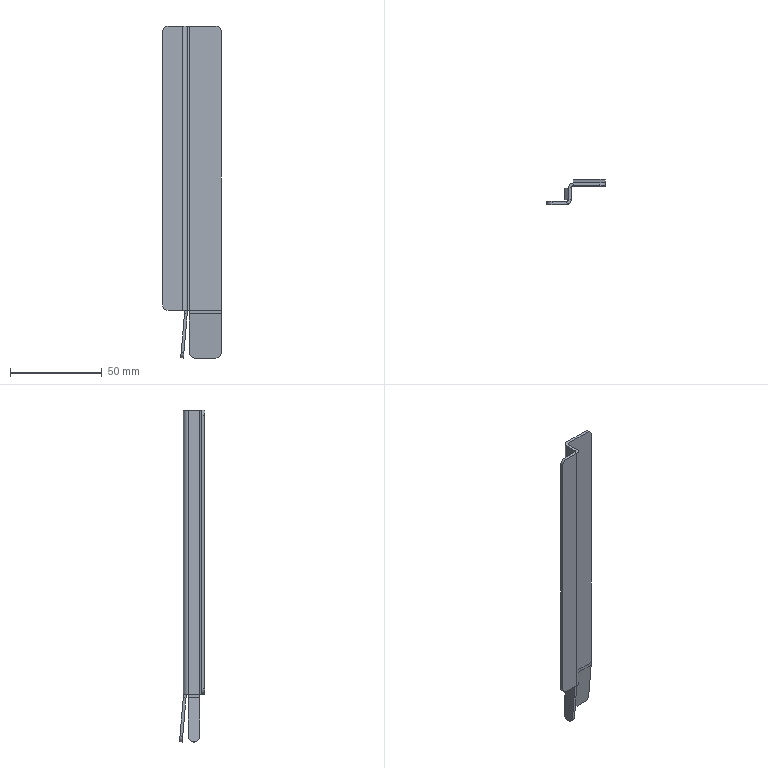Part | STEP file | 001-004-Feeding mechanism feed guide chute 2 | 1 solid | 45 faces | box 32 x 13.679 x 180.909 mm | volume 10329 mm3 | plane 30 | cylinder 15 | commonest cylinder face diameters 6 x7 2 x2 5 x2 40 x2 43 x2